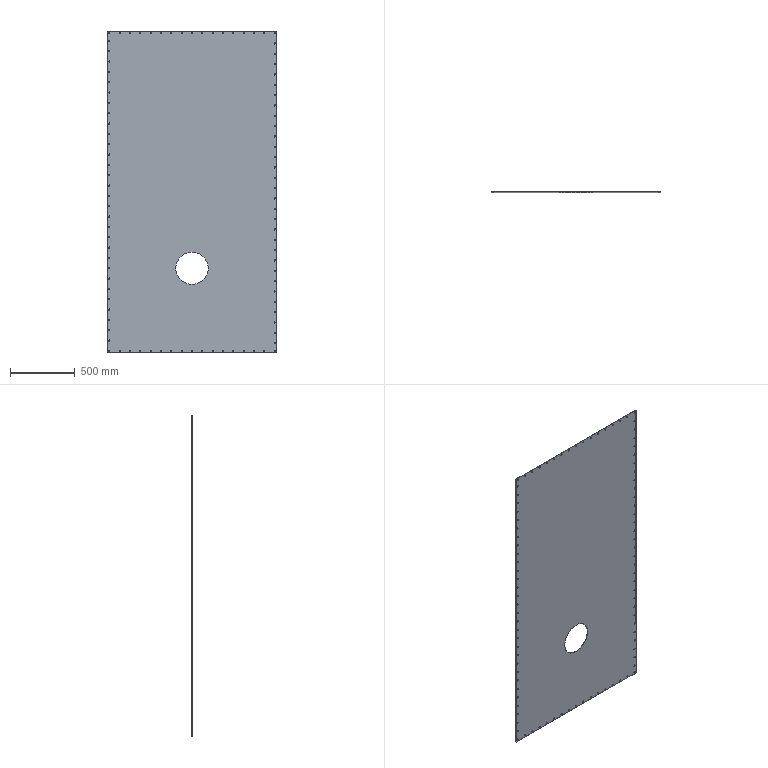Part | SolidWorks | features CirPattern 2, HoleWzd 2, LPattern 2, Extrusion 1, ICE 1, RefAxis 1 | 1 solid | 196 faces | box 1310 x 4 x 2490 mm | volume 12821719 mm3 | cylinder 190 | plane 6 | commonest cylinder face diameters 10 x188 250 x2